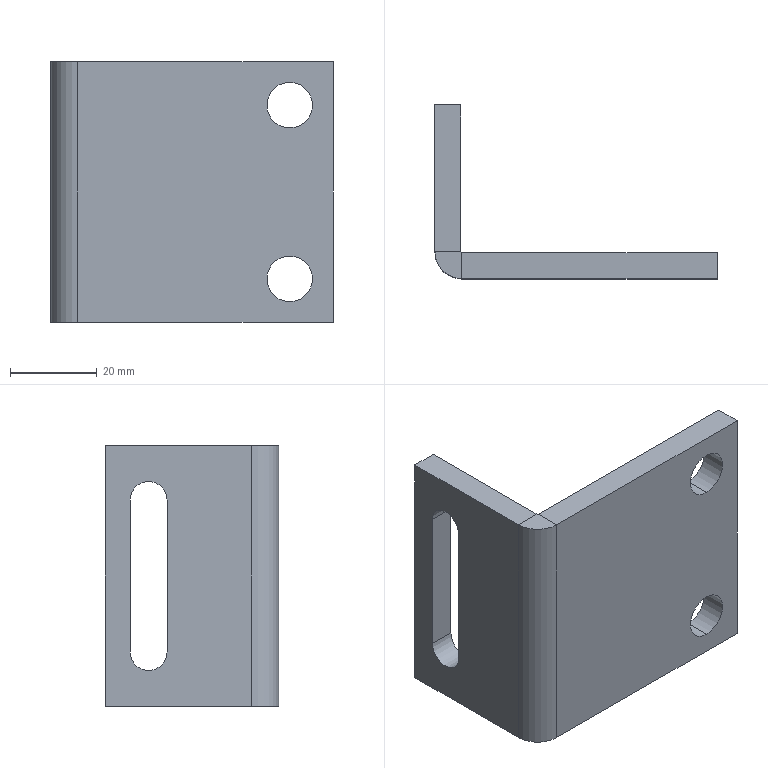Part | SolidWorks | features ICE 2, FlatPattern 1, SMBaseFlange 1, SheetMetal 1 | 1 solid | 22 faces | box 65 x 40 x 60 mm | volume 31981 mm3 | plane 14 | cylinder 8 | commonest cylinder face diameters 10.5 x4 8.5 x2 0.4 x1 12.4 x1
STEP:
#1=CARTESIAN_POINT('',(55.,0.,-25.25));
#2=VERTEX_POINT('',#1);
#3=CARTESIAN_POINT('',(55.,0.,-14.75));
#4=VERTEX_POINT('',#3);
#5=CARTESIAN_POINT('',(55.,0.,-20.));
#6=DIRECTION('',(0.,1.,0.));
#7=DIRECTION('',(0.,0.,1.));
#8=AXIS2_PLACEMENT_3D('',#5,#6,#7);
#9=CIRCLE('',#8,5.25);
#10=EDGE_CURVE('',#2,#4,#9,.T.);
#11=ORIENTED_EDGE('',*,*,#10,.F.);
#12=CARTESIAN_POINT('',(55.,6.,-25.25));
#13=VERTEX_POINT('',#12);
#14=CARTESIAN_POINT('',(55.,-4.,-25.25));
#15=DIRECTION('',(0.,1.,0.));
#16=VECTOR('',#15,1000.);
#17=LINE('',#14,#16);
#18=EDGE_CURVE('',#2,#13,#17,.T.);
#19=ORIENTED_EDGE('',*,*,#18,.T.);
#20=CARTESIAN_POINT('',(55.,6.,-14.75));
#21=VERTEX_POINT('',#20);
#22=CARTESIAN_POINT('',(55.,6.,-20.));
#23=DIRECTION('',(0.,1.,0.));
#24=DIRECTION('',(0.,0.,1.));
#25=AXIS2_PLACEMENT_3D('',#22,#23,#24);
#26=CIRCLE('',#25,5.25);
#27=EDGE_CURVE('',#13,#21,#26,.T.);
#28=ORIENTED_EDGE('',*,*,#27,.T.);
#29=CARTESIAN_POINT('',(55.,-4.,-14.75));
#30=DIRECTION('',(0.,1.,0.));
#31=VECTOR('',#30,1000.);
#32=LINE('',#29,#31);
#33=EDGE_CURVE('',#4,#21,#32,.T.);
#34=ORIENTED_EDGE('',*,*,#33,.F.);
#35=EDGE_LOOP('',(#11,#19,#28,#34));
#36=FACE_OUTER_BOUND('',#35,.T.);
#37=CARTESIAN_POINT('',(55.,-4.,-20.));
#38=DIRECTION('',(0.,1.,0.));
#39=DIRECTION('',(0.,0.,1.));
#40=AXIS2_PLACEMENT_3D('',#37,#38,#39);
#41=CYLINDRICAL_SURFACE('',#40,5.25);
#42=ADVANCED_FACE('',(#36),#41,.F.);
#43=CARTESIAN_POINT('',(55.,0.,14.75));
#44=VERTEX_POINT('',#43);
#45=CARTESIAN_POINT('',(55.,0.,25.25));
#46=VERTEX_POINT('',#45);
#47=CARTESIAN_POINT('',(55.,0.,20.));
#48=DIRECTION('',(0.,1.,0.));
#49=DIRECTION('',(0.,0.,1.));
#50=AXIS2_PLACEMENT_3D('',#47,#48,#49);
#51=CIRCLE('',#50,5.25);
#52=EDGE_CURVE('',#44,#46,#51,.T.);
#53=ORIENTED_EDGE('',*,*,#52,.F.);
#54=CARTESIAN_POINT('',(55.,6.,14.75));
#55=VERTEX_POINT('',#54);
#56=CARTESIAN_POINT('',(55.,-4.,14.75));
#57=DIRECTION('',(0.,1.,0.));
#58=VECTOR('',#57,1000.);
#59=LINE('',#56,#58);
#60=EDGE_CURVE('',#44,#55,#59,.T.);
#61=ORIENTED_EDGE('',*,*,#60,.T.);
#62=CARTESIAN_POINT('',(55.,6.,25.25));
#63=VERTEX_POINT('',#62);
#64=CARTESIAN_POINT('',(55.,6.,20.));
#65=DIRECTION('',(0.,1.,0.));
#66=DIRECTION('',(0.,0.,1.));
#67=AXIS2_PLACEMENT_3D('',#64,#65,#66);
#68=CIRCLE('',#67,5.25);
#69=EDGE_CURVE('',#55,#63,#68,.T.);
#70=ORIENTED_EDGE('',*,*,#69,.T.);
#71=CARTESIAN_POINT('',(55.,-4.,25.25));
#72=DIRECTION('',(0.,1.,0.));
#73=VECTOR('',#72,1000.);
#74=LINE('',#71,#73);
#75=EDGE_CURVE('',#46,#63,#74,.T.);
#76=ORIENTED_EDGE('',*,*,#75,.F.);
#77=EDGE_LOOP('',(#53,#61,#70,#76));
#78=FACE_OUTER_BOUND('',#77,.T.);
#79=CARTESIAN_POINT('',(55.,-4.,20.));
#80=DIRECTION('',(0.,1.,0.));
#81=DIRECTION('',(0.,0.,1.));
#82=AXIS2_PLACEMENT_3D('',#79,#80,#81);
#83=CYLINDRICAL_SURFACE('',#82,5.25);
#84=ADVANCED_FACE('',(#78),#83,.F.);
#85=CARTESIAN_POINT('',(0.,6.2,30.));
#86=VERTEX_POINT('',#85);
#87=CARTESIAN_POINT('',(6.,6.2,30.));
#88=VERTEX_POINT('',#87);
#89=CARTESIAN_POINT('',(0.,6.2,30.));
#90=DIRECTION('',(1.,0.,0.));
#91=VECTOR('',#90,1000.);
#92=LINE('',#89,#91);
#93=EDGE_CURVE('',#86,#88,#92,.T.);
#94=ORIENTED_EDGE('',*,*,#93,.F.);
#95=CARTESIAN_POINT('',(6.2,0.,30.));
#96=VERTEX_POINT('',#95);
#97=CARTESIAN_POINT('',(6.2,6.2,30.));
#98=DIRECTION('',(0.,0.,1.));
#99=DIRECTION('',(-1.,0.,0.));
#100=AXIS2_PLACEMENT_3D('',#97,#98,#99);
#101=CIRCLE('',#100,6.2);
#102=EDGE_CURVE('',#86,#96,#101,.T.);
#103=ORIENTED_EDGE('',*,*,#102,.T.);
#104=CARTESIAN_POINT('',(6.2,6.,30.));
#105=VERTEX_POINT('',#104);
#106=CARTESIAN_POINT('',(6.2,6.,30.));
#107=DIRECTION('',(0.,-1.,0.));
#108=VECTOR('',#107,1000.);
#109=LINE('',#106,#108);
#110=EDGE_CURVE('',#105,#96,#109,.T.);
#111=ORIENTED_EDGE('',*,*,#110,.F.);
#112=CARTESIAN_POINT('',(6.2,6.2,30.));
#113=DIRECTION('',(0.,0.,1.));
#114=DIRECTION('',(1.,0.,0.));
#115=AXIS2_PLACEMENT_3D('',#112,#113,#114);
#116=CIRCLE('',#115,0.2);
#117=EDGE_CURVE('',#88,#105,#116,.T.);
#118=ORIENTED_EDGE('',*,*,#117,.F.);
#119=EDGE_LOOP('',(#94,#103,#111,#118));
#120=FACE_OUTER_BOUND('',#119,.T.);
#121=CARTESIAN_POINT('',(0.,6.2,30.));
#122=DIRECTION('',(0.,0.,1.));
#123=DIRECTION('',(1.,0.,0.));
#124=AXIS2_PLACEMENT_3D('',#121,#122,#123);
#125=PLANE('',#124);
#126=ADVANCED_FACE('',(#120),#125,.T.);
#127=CARTESIAN_POINT('',(0.,40.,30.));
#128=VERTEX_POINT('',#127);
#129=CARTESIAN_POINT('',(0.,40.,30.));
#130=DIRECTION('',(0.,-1.,0.));
#131=VECTOR('',#130,1000.);
#132=LINE('',#129,#131);
#133=EDGE_CURVE('',#128,#86,#132,.T.);
#134=ORIENTED_EDGE('',*,*,#133,.T.);
#135=ORIENTED_EDGE('',*,*,#93,.T.);
#136=CARTESIAN_POINT('',(6.,40.,30.));
#137=VERTEX_POINT('',#136);
#138=CARTESIAN_POINT('',(6.,40.,30.));
#139=DIRECTION('',(0.,-1.,0.));
#140=VECTOR('',#139,1000.);
#141=LINE('',#138,#140);
#142=EDGE_CURVE('',#137,#88,#141,.T.);
#143=ORIENTED_EDGE('',*,*,#142,.F.);
#144=CARTESIAN_POINT('',(0.,40.,30.));
#145=DIRECTION('',(1.,0.,0.));
#146=VECTOR('',#145,1000.);
#147=LINE('',#144,#146);
#148=EDGE_CURVE('',#128,#137,#147,.T.);
#149=ORIENTED_EDGE('',*,*,#148,.F.);
#150=EDGE_LOOP('',(#134,#135,#143,#149));
#151=FACE_OUTER_BOUND('',#150,.T.);
#152=CARTESIAN_POINT('',(6.2,6.,30.));
#153=DIRECTION('',(0.,0.,1.));
#154=DIRECTION('',(1.,0.,0.));
#155=AXIS2_PLACEMENT_3D('',#152,#153,#154);
#156=PLANE('',#155);
#157=ADVANCED_FACE('',(#151),#156,.T.);
#158=CARTESIAN_POINT('',(6.2,0.,-30.));
#159=VERTEX_POINT('',#158);
#160=CARTESIAN_POINT('',(6.2,6.,-30.));
#161=VERTEX_POINT('',#160);
#162=CARTESIAN_POINT('',(6.2,0.,-30.));
#163=DIRECTION('',(0.,1.,0.));
#164=VECTOR('',#163,1000.);
#165=LINE('',#162,#164);
#166=EDGE_CURVE('',#159,#161,#165,.T.);
#167=ORIENTED_EDGE('',*,*,#166,.F.);
#168=CARTESIAN_POINT('',(0.,6.2,-30.));
#169=VERTEX_POINT('',#168);
#170=CARTESIAN_POINT('',(6.2,6.2,-30.));
#171=DIRECTION('',(0.,0.,1.));
#172=DIRECTION('',(-1.,0.,0.));
#173=AXIS2_PLACEMENT_3D('',#170,#171,#172);
#174=CIRCLE('',#173,6.2);
#175=EDGE_CURVE('',#169,#159,#174,.T.);
#176=ORIENTED_EDGE('',*,*,#175,.F.);
#177=CARTESIAN_POINT('',(6.,6.2,-30.));
#178=VERTEX_POINT('',#177);
#179=CARTESIAN_POINT('',(6.,6.2,-30.));
#180=DIRECTION('',(-1.,0.,0.));
#181=VECTOR('',#180,1000.);
#182=LINE('',#179,#181);
#183=EDGE_CURVE('',#178,#169,#182,.T.);
#184=ORIENTED_EDGE('',*,*,#183,.F.);
#185=CARTESIAN_POINT('',(6.2,6.2,-30.));
#186=DIRECTION('',(0.,0.,1.));
#187=DIRECTION('',(1.,0.,0.));
#188=AXIS2_PLACEMENT_3D('',#185,#186,#187);
#189=CIRCLE('',#188,0.2);
#190=EDGE_CURVE('',#178,#161,#189,.T.);
#191=ORIENTED_EDGE('',*,*,#190,.T.);
#192=EDGE_LOOP('',(#167,#176,#184,#191));
#193=FACE_OUTER_BOUND('',#192,.T.);
#194=CARTESIAN_POINT('',(6.2,0.,-30.));
#195=DIRECTION('',(0.,0.,-1.));
#196=DIRECTION('',(-1.,0.,0.));
#197=AXIS2_PLACEMENT_3D('',#194,#195,#196);
#198=PLANE('',#197);
#199=ADVANCED_FACE('',(#193),#198,.T.);
#200=CARTESIAN_POINT('',(65.,0.,-30.));
#201=VERTEX_POINT('',#200);
#202=CARTESIAN_POINT('',(0.,0.,-30.));
#203=DIRECTION('',(1.,0.,0.));
#204=VECTOR('',#203,1000.);
#205=LINE('',#202,#204);
#206=EDGE_CURVE('',#159,#201,#205,.T.);
#207=ORIENTED_EDGE('',*,*,#206,.F.);
#208=ORIENTED_EDGE('',*,*,#166,.T.);
#209=CARTESIAN_POINT('',(65.,6.,-30.));
#210=VERTEX_POINT('',#209);
#211=CARTESIAN_POINT('',(0.,6.,-30.));
#212=DIRECTION('',(1.,0.,0.));
#213=VECTOR('',#212,1000.);
#214=LINE('',#211,#213);
#215=EDGE_CURVE('',#161,#210,#214,.T.);
#216=ORIENTED_EDGE('',*,*,#215,.T.);
#217=CARTESIAN_POINT('',(65.,6.,-30.));
#218=DIRECTION('',(0.,-1.,0.));
#219=VECTOR('',#218,1000.);
#220=LINE('',#217,#219);
#221=EDGE_CURVE('',#210,#201,#220,.T.);
#222=ORIENTED_EDGE('',*,*,#221,.T.);
#223=EDGE_LOOP('',(#207,#208,#216,#222));
#224=FACE_OUTER_BOUND('',#223,.T.);
#225=CARTESIAN_POINT('',(6.,6.2,-30.));
#226=DIRECTION('',(0.,0.,-1.));
#227=DIRECTION('',(-1.,0.,0.));
#228=AXIS2_PLACEMENT_3D('',#225,#226,#227);
#229=PLANE('',#228);
#230=ADVANCED_FACE('',(#224),#229,.T.);
#231=CARTESIAN_POINT('',(55.,0.,-20.));
#232=DIRECTION('',(0.,1.,0.));
#233=DIRECTION('',(0.,0.,1.));
#234=AXIS2_PLACEMENT_3D('',#231,#232,#233);
#235=CIRCLE('',#234,5.25);
#236=EDGE_CURVE('',#4,#2,#235,.T.);
#237=ORIENTED_EDGE('',*,*,#236,.T.);
#238=ORIENTED_EDGE('',*,*,#10,.T.);
#239=EDGE_LOOP('',(#237,#238));
#240=FACE_BOUND('',#239,.T.);
#241=CARTESIAN_POINT('',(55.,0.,20.));
#242=DIRECTION('',(0.,1.,0.));
#243=DIRECTION('',(0.,0.,1.));
#244=AXIS2_PLACEMENT_3D('',#241,#242,#243);
#245=CIRCLE('',#244,5.25);
#246=EDGE_CURVE('',#46,#44,#245,.T.);
#247=ORIENTED_EDGE('',*,*,#246,.T.);
#248=ORIENTED_EDGE('',*,*,#52,.T.);
#249=EDGE_LOOP('',(#247,#248));
#250=FACE_BOUND('',#249,.T.);
#251=ORIENTED_EDGE('',*,*,#206,.T.);
#252=CARTESIAN_POINT('',(65.,0.,30.));
#253=VERTEX_POINT('',#252);
#254=CARTESIAN_POINT('',(65.,0.,30.));
#255=DIRECTION('',(0.,0.,-1.));
#256=VECTOR('',#255,1000.);
#257=LINE('',#254,#256);
#258=EDGE_CURVE('',#253,#201,#257,.T.);
#259=ORIENTED_EDGE('',*,*,#258,.F.);
#260=CARTESIAN_POINT('',(0.,0.,30.));
#261=DIRECTION('',(1.,0.,0.));
#262=VECTOR('',#261,1000.);
#263=LINE('',#260,#262);
#264=EDGE_CURVE('',#96,#253,#263,.T.);
#265=ORIENTED_EDGE('',*,*,#264,.F.);
#266=CARTESIAN_POINT('',(6.2,0.,30.));
#267=DIRECTION('',(0.,0.,-1.));
#268=VECTOR('',#267,1000.);
#269=LINE('',#266,#268);
#270=EDGE_CURVE('',#96,#159,#269,.T.);
#271=ORIENTED_EDGE('',*,*,#270,.T.);
#272=EDGE_LOOP('',(#251,#259,#265,#271));
#273=FACE_OUTER_BOUND('',#272,.T.);
#274=CARTESIAN_POINT('',(0.,0.,30.));
#275=DIRECTION('',(0.,1.,0.));
#276=DIRECTION('',(0.,0.,1.));
#277=AXIS2_PLACEMENT_3D('',#274,#275,#276);
#278=PLANE('',#277);
#279=ADVANCED_FACE('',(#240,#250,#273),#278,.F.);
#280=ORIENTED_EDGE('',*,*,#221,.F.);
#281=CARTESIAN_POINT('',(65.,6.,30.));
#282=VERTEX_POINT('',#281);
#283=CARTESIAN_POINT('',(65.,6.,30.));
#284=DIRECTION('',(0.,0.,-1.));
#285=VECTOR('',#284,1000.);
#286=LINE('',#283,#285);
#287=EDGE_CURVE('',#282,#210,#286,.T.);
#288=ORIENTED_EDGE('',*,*,#287,.F.);
#289=CARTESIAN_POINT('',(65.,6.,30.));
#290=DIRECTION('',(0.,-1.,0.));
#291=VECTOR('',#290,1000.);
#292=LINE('',#289,#291);
#293=EDGE_CURVE('',#282,#253,#292,.T.);
#294=ORIENTED_EDGE('',*,*,#293,.T.);
#295=ORIENTED_EDGE('',*,*,#258,.T.);
#296=EDGE_LOOP('',(#280,#288,#294,#295));
#297=FACE_OUTER_BOUND('',#296,.T.);
#298=CARTESIAN_POINT('',(65.,6.,30.));
#299=DIRECTION('',(1.,0.,0.));
#300=DIRECTION('',(0.,0.,-1.));
#301=AXIS2_PLACEMENT_3D('',#298,#299,#300);
#302=PLANE('',#301);
#303=ADVANCED_FACE('',(#297),#302,.T.);
#304=CARTESIAN_POINT('',(55.,6.,-20.));
#305=DIRECTION('',(0.,1.,0.));
#306=DIRECTION('',(0.,0.,1.));
#307=AXIS2_PLACEMENT_3D('',#304,#305,#306);
#308=CIRCLE('',#307,5.25);
#309=EDGE_CURVE('',#21,#13,#308,.T.);
#310=ORIENTED_EDGE('',*,*,#309,.F.);
#311=ORIENTED_EDGE('',*,*,#27,.F.);
#312=EDGE_LOOP('',(#310,#311));
#313=FACE_BOUND('',#312,.T.);
#314=CARTESIAN_POINT('',(55.,6.,20.));
#315=DIRECTION('',(0.,1.,0.));
#316=DIRECTION('',(0.,0.,1.));
#317=AXIS2_PLACEMENT_3D('',#314,#315,#316);
#318=CIRCLE('',#317,5.25);
#319=EDGE_CURVE('',#63,#55,#318,.T.);
#320=ORIENTED_EDGE('',*,*,#319,.F.);
#321=ORIENTED_EDGE('',*,*,#69,.F.);
#322=EDGE_LOOP('',(#320,#321));
#323=FACE_BOUND('',#322,.T.);
#324=ORIENTED_EDGE('',*,*,#215,.F.);
#325=CARTESIAN_POINT('',(6.2,6.,30.));
#326=DIRECTION('',(0.,0.,-1.));
#327=VECTOR('',#326,1000.);
#328=LINE('',#325,#327);
#329=EDGE_CURVE('',#105,#161,#328,.T.);
#330=ORIENTED_EDGE('',*,*,#329,.F.);
#331=CARTESIAN_POINT('',(0.,6.,30.));
#332=DIRECTION('',(1.,0.,0.));
#333=VECTOR('',#332,1000.);
#334=LINE('',#331,#333);
#335=EDGE_CURVE('',#105,#282,#334,.T.);
#336=ORIENTED_EDGE('',*,*,#335,.T.);
#337=ORIENTED_EDGE('',*,*,#287,.T.);
#338=EDGE_LOOP('',(#324,#330,#336,#337));
#339=FACE_OUTER_BOUND('',#338,.T.);
#340=CARTESIAN_POINT('',(0.,6.,30.));
#341=DIRECTION('',(0.,1.,0.));
#342=DIRECTION('',(0.,0.,1.));
#343=AXIS2_PLACEMENT_3D('',#340,#341,#342);
#344=PLANE('',#343);
#345=ADVANCED_FACE('',(#313,#323,#339),#344,.T.);
#346=ORIENTED_EDGE('',*,*,#190,.F.);
#347=CARTESIAN_POINT('',(6.,6.2,30.));
#348=DIRECTION('',(0.,0.,-1.));
#349=VECTOR('',#348,1000.);
#350=LINE('',#347,#349);
#351=EDGE_CURVE('',#88,#178,#350,.T.);
#352=ORIENTED_EDGE('',*,*,#351,.F.);
#353=ORIENTED_EDGE('',*,*,#117,.T.);
#354=ORIENTED_EDGE('',*,*,#329,.T.);
#355=EDGE_LOOP('',(#346,#352,#353,#354));
#356=FACE_OUTER_BOUND('',#355,.T.);
#357=CARTESIAN_POINT('',(6.2,6.2,30.));
#358=DIRECTION('',(0.,0.,-1.));
#359=DIRECTION('',(-1.,0.,0.));
#360=AXIS2_PLACEMENT_3D('',#357,#358,#359);
#361=CYLINDRICAL_SURFACE('',#360,0.2);
#362=ADVANCED_FACE('',(#356),#361,.F.);
#363=CARTESIAN_POINT('',(6.,34.25,17.5));
#364=VERTEX_POINT('',#363);
#365=CARTESIAN_POINT('',(6.,25.75,17.5));
#366=VERTEX_POINT('',#365);
#367=CARTESIAN_POINT('',(6.,30.,17.5));
#368=DIRECTION('',(1.,0.,0.));
#369=DIRECTION('',(0.,1.,0.));
#370=AXIS2_PLACEMENT_3D('',#367,#368,#369);
#371=CIRCLE('',#370,4.25);
#372=EDGE_CURVE('',#364,#366,#371,.T.);
#373=ORIENTED_EDGE('',*,*,#372,.F.);
#374=CARTESIAN_POINT('',(6.,34.25,-17.5));
#375=VERTEX_POINT('',#374);
#376=CARTESIAN_POINT('',(6.,34.25,17.5));
#377=DIRECTION('',(0.,0.,1.));
#378=VECTOR('',#377,1000.);
#379=LINE('',#376,#378);
#380=EDGE_CURVE('',#375,#364,#379,.T.);
#381=ORIENTED_EDGE('',*,*,#380,.F.);
#382=CARTESIAN_POINT('',(6.,25.75,-17.5));
#383=VERTEX_POINT('',#382);
#384=CARTESIAN_POINT('',(6.,30.,-17.5));
#385=DIRECTION('',(1.,0.,0.));
#386=DIRECTION('',(0.,1.,0.));
#387=AXIS2_PLACEMENT_3D('',#384,#385,#386);
#388=CIRCLE('',#387,4.25);
#389=EDGE_CURVE('',#383,#375,#388,.T.);
#390=ORIENTED_EDGE('',*,*,#389,.F.);
#391=CARTESIAN_POINT('',(6.,25.75,17.5));
#392=DIRECTION('',(0.,0.,-1.));
#393=VECTOR('',#392,1000.);
#394=LINE('',#391,#393);
#395=EDGE_CURVE('',#366,#383,#394,.T.);
#396=ORIENTED_EDGE('',*,*,#395,.F.);
#397=EDGE_LOOP('',(#373,#381,#390,#396));
#398=FACE_BOUND('',#397,.T.);
#399=CARTESIAN_POINT('',(6.,40.,-30.));
#400=VERTEX_POINT('',#399);
#401=CARTESIAN_POINT('',(6.,40.,-30.));
#402=DIRECTION('',(0.,-1.,0.));
#403=VECTOR('',#402,1000.);
#404=LINE('',#401,#403);
#405=EDGE_CURVE('',#400,#178,#404,.T.);
#406=ORIENTED_EDGE('',*,*,#405,.F.);
#407=CARTESIAN_POINT('',(6.,40.,30.));
#408=DIRECTION('',(0.,0.,-1.));
#409=VECTOR('',#408,1000.);
#410=LINE('',#407,#409);
#411=EDGE_CURVE('',#137,#400,#410,.T.);
#412=ORIENTED_EDGE('',*,*,#411,.F.);
#413=ORIENTED_EDGE('',*,*,#142,.T.);
#414=ORIENTED_EDGE('',*,*,#351,.T.);
#415=EDGE_LOOP('',(#406,#412,#413,#414));
#416=FACE_OUTER_BOUND('',#415,.T.);
#417=CARTESIAN_POINT('',(6.,40.,30.));
#418=DIRECTION('',(1.,0.,0.));
#419=DIRECTION('',(0.,1.,0.));
#420=AXIS2_PLACEMENT_3D('',#417,#418,#419);
#421=PLANE('',#420);
#422=ADVANCED_FACE('',(#398,#416),#421,.T.);
#423=CARTESIAN_POINT('',(0.,40.,-30.));
#424=VERTEX_POINT('',#423);
#425=CARTESIAN_POINT('',(0.,40.,-30.));
#426=DIRECTION('',(1.,0.,0.));
#427=VECTOR('',#426,1000.);
#428=LINE('',#425,#427);
#429=EDGE_CURVE('',#424,#400,#428,.T.);
#430=ORIENTED_EDGE('',*,*,#429,.F.);
#431=CARTESIAN_POINT('',(0.,40.,30.));
#432=DIRECTION('',(0.,0.,-1.));
#433=VECTOR('',#432,1000.);
#434=LINE('',#431,#433);
#435=EDGE_CURVE('',#128,#424,#434,.T.);
#436=ORIENTED_EDGE('',*,*,#435,.F.);
#437=ORIENTED_EDGE('',*,*,#148,.T.);
#438=ORIENTED_EDGE('',*,*,#411,.T.);
#439=EDGE_LOOP('',(#430,#436,#437,#438));
#440=FACE_OUTER_BOUND('',#439,.T.);
#441=CARTESIAN_POINT('',(0.,40.,30.));
#442=DIRECTION('',(0.,1.,0.));
#443=DIRECTION('',(0.,0.,1.));
#444=AXIS2_PLACEMENT_3D('',#441,#442,#443);
#445=PLANE('',#444);
#446=ADVANCED_FACE('',(#440),#445,.T.);
#447=CARTESIAN_POINT('',(0.,34.25,-17.5));
#448=VERTEX_POINT('',#447);
#449=CARTESIAN_POINT('',(0.,34.25,17.5));
#450=VERTEX_POINT('',#449);
#451=CARTESIAN_POINT('',(0.,34.25,30.));
#452=DIRECTION('',(0.,0.,1.));
#453=VECTOR('',#452,1000.);
#454=LINE('',#451,#453);
#455=EDGE_CURVE('',#448,#450,#454,.T.);
#456=ORIENTED_EDGE('',*,*,#455,.T.);
#457=CARTESIAN_POINT('',(0.,25.75,17.5));
#458=VERTEX_POINT('',#457);
#459=CARTESIAN_POINT('',(0.,30.,17.5));
#460=DIRECTION('',(1.,0.,0.));
#461=DIRECTION('',(0.,1.,0.));
#462=AXIS2_PLACEMENT_3D('',#459,#460,#461);
#463=CIRCLE('',#462,4.25);
#464=EDGE_CURVE('',#450,#458,#463,.T.);
#465=ORIENTED_EDGE('',*,*,#464,.T.);
#466=CARTESIAN_POINT('',(0.,25.75,-17.5));
#467=VERTEX_POINT('',#466);
#468=CARTESIAN_POINT('',(0.,25.75,30.));
#469=DIRECTION('',(0.,0.,-1.));
#470=VECTOR('',#469,1000.);
#471=LINE('',#468,#470);
#472=EDGE_CURVE('',#458,#467,#471,.T.);
#473=ORIENTED_EDGE('',*,*,#472,.T.);
#474=CARTESIAN_POINT('',(0.,30.,-17.5));
#475=DIRECTION('',(1.,0.,0.));
#476=DIRECTION('',(0.,1.,0.));
#477=AXIS2_PLACEMENT_3D('',#474,#475,#476);
#478=CIRCLE('',#477,4.25);
#479=EDGE_CURVE('',#467,#448,#478,.T.);
#480=ORIENTED_EDGE('',*,*,#479,.T.);
#481=EDGE_LOOP('',(#456,#465,#473,#480));
#482=FACE_BOUND('',#481,.T.);
#483=CARTESIAN_POINT('',(0.,40.,-30.));
#484=DIRECTION('',(0.,-1.,0.));
#485=VECTOR('',#484,1000.);
#486=LINE('',#483,#485);
#487=EDGE_CURVE('',#424,#169,#486,.T.);
#488=ORIENTED_EDGE('',*,*,#487,.T.);
#489=CARTESIAN_POINT('',(0.,6.2,30.));
#490=DIRECTION('',(0.,0.,-1.));
#491=VECTOR('',#490,1000.);
#492=LINE('',#489,#491);
#493=EDGE_CURVE('',#86,#169,#492,.T.);
#494=ORIENTED_EDGE('',*,*,#493,.F.);
#495=ORIENTED_EDGE('',*,*,#133,.F.);
#496=ORIENTED_EDGE('',*,*,#435,.T.);
#497=EDGE_LOOP('',(#488,#494,#495,#496));
#498=FACE_OUTER_BOUND('',#497,.T.);
#499=CARTESIAN_POINT('',(0.,40.,30.));
#500=DIRECTION('',(1.,0.,0.));
#501=DIRECTION('',(0.,1.,0.));
#502=AXIS2_PLACEMENT_3D('',#499,#500,#501);
#503=PLANE('',#502);
#504=ADVANCED_FACE('',(#482,#498),#503,.F.);
#505=ORIENTED_EDGE('',*,*,#175,.T.);
#506=ORIENTED_EDGE('',*,*,#270,.F.);
#507=ORIENTED_EDGE('',*,*,#102,.F.);
#508=ORIENTED_EDGE('',*,*,#493,.T.);
#509=EDGE_LOOP('',(#505,#506,#507,#508));
#510=FACE_OUTER_BOUND('',#509,.T.);
#511=CARTESIAN_POINT('',(6.2,6.2,30.));
#512=DIRECTION('',(0.,0.,-1.));
#513=DIRECTION('',(-1.,0.,0.));
#514=AXIS2_PLACEMENT_3D('',#511,#512,#513);
#515=CYLINDRICAL_SURFACE('',#514,6.2);
#516=ADVANCED_FACE('',(#510),#515,.T.);
#517=ORIENTED_EDGE('',*,*,#264,.T.);
#518=ORIENTED_EDGE('',*,*,#293,.F.);
#519=ORIENTED_EDGE('',*,*,#335,.F.);
#520=ORIENTED_EDGE('',*,*,#110,.T.);
#521=EDGE_LOOP('',(#517,#518,#519,#520));
#522=FACE_OUTER_BOUND('',#521,.T.);
#523=CARTESIAN_POINT('',(6.2,6.2,30.));
#524=DIRECTION('',(0.,0.,1.));
#525=DIRECTION('',(1.,0.,0.));
#526=AXIS2_PLACEMENT_3D('',#523,#524,#525);
#527=PLANE('',#526);
#528=ADVANCED_FACE('',(#522),#527,.T.);
#529=ORIENTED_EDGE('',*,*,#405,.T.);
#530=ORIENTED_EDGE('',*,*,#183,.T.);
#531=ORIENTED_EDGE('',*,*,#487,.F.);
#532=ORIENTED_EDGE('',*,*,#429,.T.);
#533=EDGE_LOOP('',(#529,#530,#531,#532));
#534=FACE_OUTER_BOUND('',#533,.T.);
#535=CARTESIAN_POINT('',(6.2,6.2,-30.));
#536=DIRECTION('',(0.,0.,1.));
#537=DIRECTION('',(1.,0.,0.));
#538=AXIS2_PLACEMENT_3D('',#535,#536,#537);
#539=PLANE('',#538);
#540=ADVANCED_FACE('',(#534),#539,.F.);
#541=CARTESIAN_POINT('',(-4.,34.25,17.5));
#542=DIRECTION('',(1.,0.,0.));
#543=VECTOR('',#542,1000.);
#544=LINE('',#541,#543);
#545=EDGE_CURVE('',#450,#364,#544,.T.);
#546=ORIENTED_EDGE('',*,*,#545,.T.);
#547=ORIENTED_EDGE('',*,*,#372,.T.);
#548=CARTESIAN_POINT('',(-4.,25.75,17.5));
#549=DIRECTION('',(1.,0.,0.));
#550=VECTOR('',#549,1000.);
#551=LINE('',#548,#550);
#552=EDGE_CURVE('',#458,#366,#551,.T.);
#553=ORIENTED_EDGE('',*,*,#552,.F.);
#554=ORIENTED_EDGE('',*,*,#464,.F.);
#555=EDGE_LOOP('',(#546,#547,#553,#554));
#556=FACE_OUTER_BOUND('',#555,.T.);
#557=CARTESIAN_POINT('',(-4.,30.,17.5));
#558=DIRECTION('',(1.,0.,0.));
#559=DIRECTION('',(0.,1.,0.));
#560=AXIS2_PLACEMENT_3D('',#557,#558,#559);
#561=CYLINDRICAL_SURFACE('',#560,4.25);
#562=ADVANCED_FACE('',(#556),#561,.F.);
#563=CARTESIAN_POINT('',(-4.,34.25,-17.5));
#564=DIRECTION('',(1.,0.,0.));
#565=VECTOR('',#564,1000.);
#566=LINE('',#563,#565);
#567=EDGE_CURVE('',#448,#375,#566,.T.);
#568=ORIENTED_EDGE('',*,*,#567,.T.);
#569=ORIENTED_EDGE('',*,*,#380,.T.);
#570=ORIENTED_EDGE('',*,*,#545,.F.);
#571=ORIENTED_EDGE('',*,*,#455,.F.);
#572=EDGE_LOOP('',(#568,#569,#570,#571));
#573=FACE_OUTER_BOUND('',#572,.T.);
#574=CARTESIAN_POINT('',(-4.,34.25,17.5));
#575=DIRECTION('',(0.,1.,0.));
#576=DIRECTION('',(0.,0.,1.));
#577=AXIS2_PLACEMENT_3D('',#574,#575,#576);
#578=PLANE('',#577);
#579=ADVANCED_FACE('',(#573),#578,.F.);
#580=CARTESIAN_POINT('',(-4.,25.75,-17.5));
#581=DIRECTION('',(1.,0.,0.));
#582=VECTOR('',#581,1000.);
#583=LINE('',#580,#582);
#584=EDGE_CURVE('',#467,#383,#583,.T.);
#585=ORIENTED_EDGE('',*,*,#584,.T.);
#586=ORIENTED_EDGE('',*,*,#389,.T.);
#587=ORIENTED_EDGE('',*,*,#567,.F.);
#588=ORIENTED_EDGE('',*,*,#479,.F.);
#589=EDGE_LOOP('',(#585,#586,#587,#588));
#590=FACE_OUTER_BOUND('',#589,.T.);
#591=CARTESIAN_POINT('',(-4.,30.,-17.5));
#592=DIRECTION('',(1.,0.,0.));
#593=DIRECTION('',(0.,1.,0.));
#594=AXIS2_PLACEMENT_3D('',#591,#592,#593);
#595=CYLINDRICAL_SURFACE('',#594,4.25);
#596=ADVANCED_FACE('',(#590),#595,.F.);
#597=ORIENTED_EDGE('',*,*,#552,.T.);
#598=ORIENTED_EDGE('',*,*,#395,.T.);
#599=ORIENTED_EDGE('',*,*,#584,.F.);
#600=ORIENTED_EDGE('',*,*,#472,.F.);
#601=EDGE_LOOP('',(#597,#598,#599,#600));
#602=FACE_OUTER_BOUND('',#601,.T.);
#603=CARTESIAN_POINT('',(-4.,25.75,17.5));
#604=DIRECTION('',(0.,-1.,0.));
#605=DIRECTION('',(0.,0.,-1.));
#606=AXIS2_PLACEMENT_3D('',#603,#604,#605);
#607=PLANE('',#606);
#608=ADVANCED_FACE('',(#602),#607,.F.);
#609=ORIENTED_EDGE('',*,*,#60,.F.);
#610=ORIENTED_EDGE('',*,*,#246,.F.);
#611=ORIENTED_EDGE('',*,*,#75,.T.);
#612=ORIENTED_EDGE('',*,*,#319,.T.);
#613=EDGE_LOOP('',(#609,#610,#611,#612));
#614=FACE_OUTER_BOUND('',#613,.T.);
#615=CARTESIAN_POINT('',(55.,-4.,20.));
#616=DIRECTION('',(0.,1.,0.));
#617=DIRECTION('',(0.,0.,1.));
#618=AXIS2_PLACEMENT_3D('',#615,#616,#617);
#619=CYLINDRICAL_SURFACE('',#618,5.25);
#620=ADVANCED_FACE('',(#614),#619,.F.);
#621=ORIENTED_EDGE('',*,*,#18,.F.);
#622=ORIENTED_EDGE('',*,*,#236,.F.);
#623=ORIENTED_EDGE('',*,*,#33,.T.);
#624=ORIENTED_EDGE('',*,*,#309,.T.);
#625=EDGE_LOOP('',(#621,#622,#623,#624));
#626=FACE_OUTER_BOUND('',#625,.T.);
#627=CARTESIAN_POINT('',(55.,-4.,-20.));
#628=DIRECTION('',(0.,1.,0.));
#629=DIRECTION('',(0.,0.,1.));
#630=AXIS2_PLACEMENT_3D('',#627,#628,#629);
#631=CYLINDRICAL_SURFACE('',#630,5.25);
#632=ADVANCED_FACE('',(#626),#631,.F.);
#633=CLOSED_SHELL('',(#42,#84,#126,#157,#199,#230,#279,#303,#345,#362,#422,#446,#504,#516,#528,#540,#562,#579,#596,#608,#620,#632));
#634=MANIFOLD_SOLID_BREP('',#633);
#635=CARTESIAN_POINT('',(0.,0.,0.));
#636=DIRECTION('',(0.,0.,1.));
#637=DIRECTION('',(1.,0.,0.));
#638=AXIS2_PLACEMENT_3D('',#635,#636,#637);
#639=(LENGTH_UNIT()NAMED_UNIT(*)SI_UNIT(.MILLI.,.METRE.));
#640=UNCERTAINTY_MEASURE_WITH_UNIT(LENGTH_MEASURE(0.00001),#639,'','');
#641=(NAMED_UNIT(*)PLANE_ANGLE_UNIT()SI_UNIT($,.RADIAN.));
#642=(NAMED_UNIT(*)SI_UNIT($,.STERADIAN.)SOLID_ANGLE_UNIT());
#643=(GEOMETRIC_REPRESENTATION_CONTEXT(3)GLOBAL_UNCERTAINTY_ASSIGNED_CONTEXT((#640))GLOBAL_UNIT_ASSIGNED_CONTEXT((#639,#641,#642))REPRESENTATION_CONTEXT('',''));
#644=ADVANCED_BREP_SHAPE_REPRESENTATION('',(#634,#638),#643);